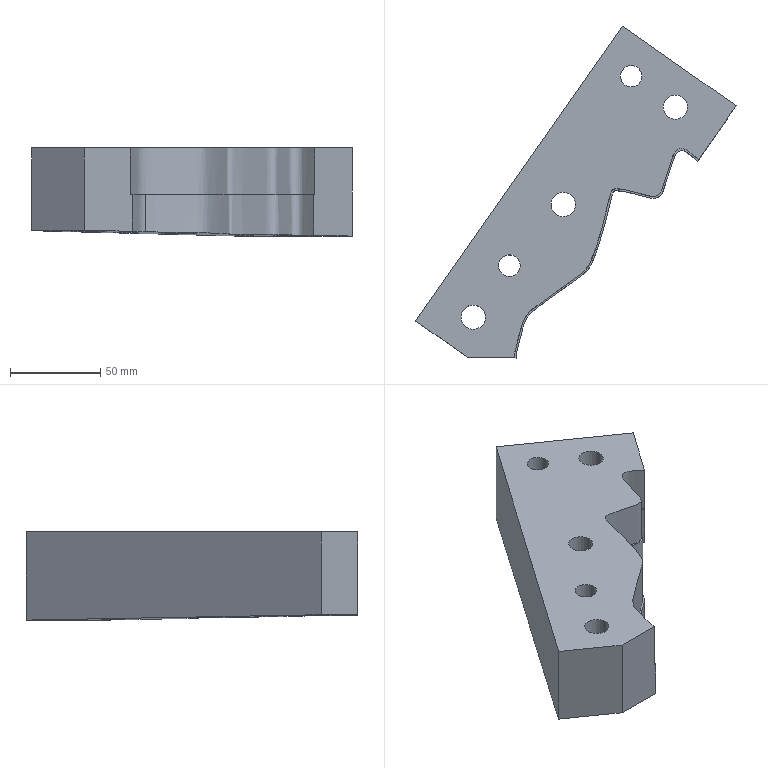Part | NX | features solid 2 | 1 solid | 26 faces | box 178.021 x 184.327 x 49 mm | volume 541406 mm3 | plane 13 | cylinder 10 | spline 3 | commonest cylinder face diameters 13.5 x3 19.5 x3 12 x2 13 x2